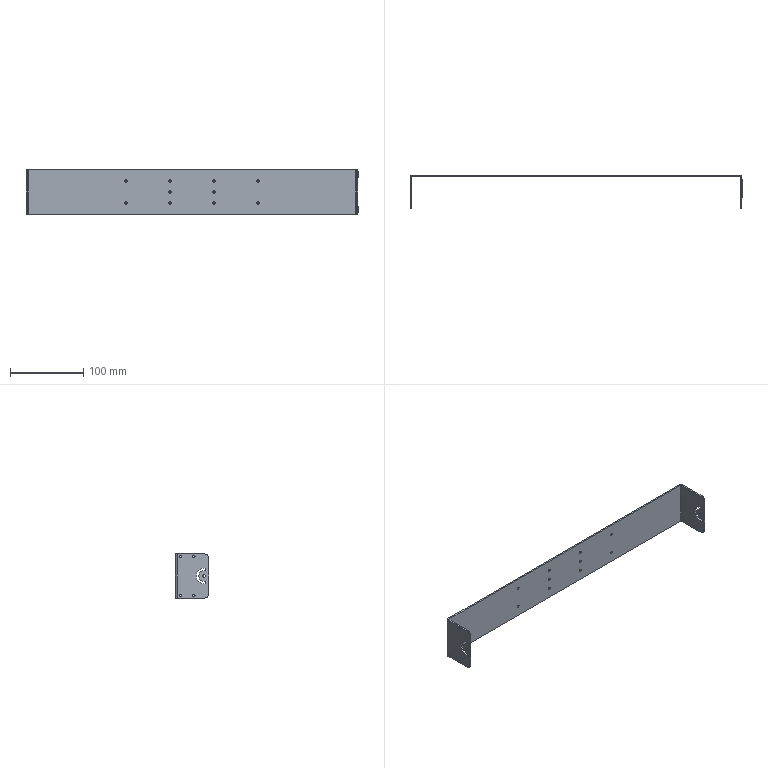Part | SolidWorks | features HoleWzd 2, ICE 2, EdgeFlange 1, Fillet 1, FlatPattern 1, SMBaseFlange 1, SheetMetal 1 | 1 solid | 74 faces | box 452 x 45 x 60 mm | volume 63539 mm3 | cylinder 52 | plane 22 | commonest cylinder face diameters 3.3 x36 3.5 x4 10 x4 1.473 x2 5.473 x2 14.5 x2